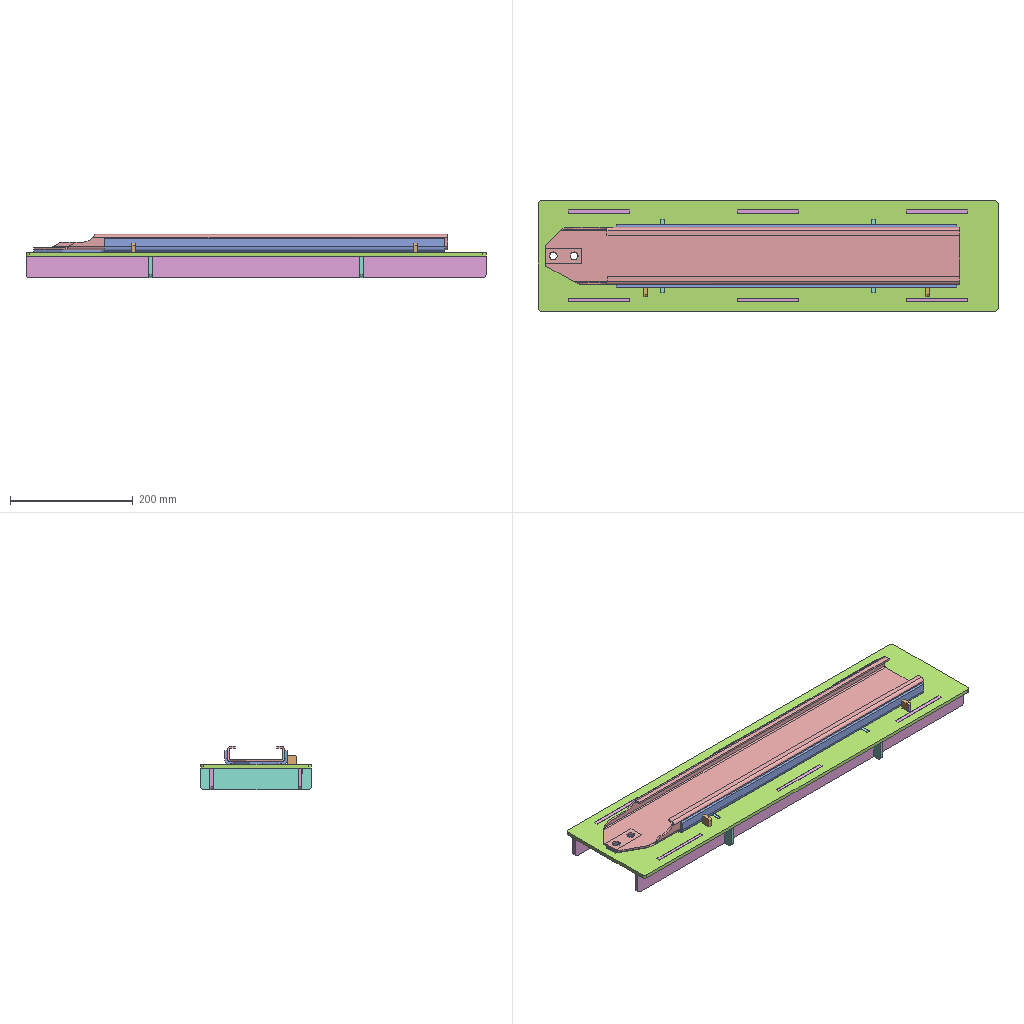Assembly | SolidWorks | 7 different items | 10 placed | box 750 x 180 x 70 mm
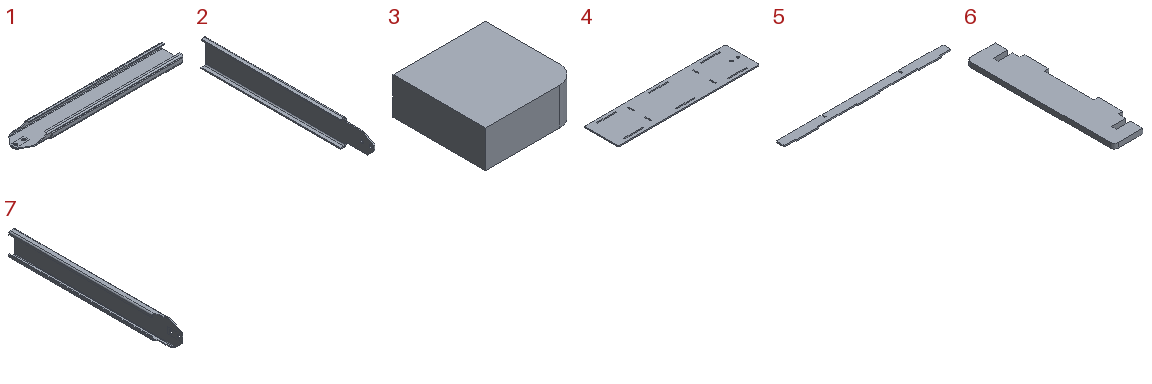Parts list (item | name | quantity | parent item | size | volume | features):
1 | (subassembly) | x1 | - | 675 x 102.2 x 29.4 mm | 664944 mm3 | -
2 | - | x1 | in 1 | 22.5 x 670 x 102.2 mm | 361914 mm3 | features ICE 2, FlatPattern 1, SMBaseFlange 1, SheetMetal 1
3 | - | x2 | - | 15 x 15 x 6 mm | 1338 mm3 | features FlatPattern 1, SMBaseFlange 1, SheetMetal 1
4 | - | x1 | - | 750 x 180 x 6 mm | 782502 mm3 | features FlatPattern 1, SMBaseFlange 1, SheetMetal 1
5 | - | x2 | - | 750 x 40.5 x 6 mm | 166068 mm3 | features FlatPattern 1, SMBaseFlange 1, SheetMetal 1
6 | - | x2 | - | 40.5 x 180 x 6 mm | 38456 mm3 | features FlatPattern 1, SMBaseFlange 1, SheetMetal 1
7 | - | x1 | in 1 | 24.9 x 675 x 92.9 mm | 303030 mm3 | features ICE 4, FlatPattern 1, SMBaseFlange 1, SheetMetal 1
Mates (type | each side: item.copy, entity, surface, feature):
In the top assembly
InPlace | 5.1 plane | assembly plane
InPlace | 6.1 plane | assembly plane
In subassembly 1
Coincident | 7.1 face plane Base-Flange1 | 2.1 face plane Base-Flange1 | 2 times
Concentric | 7.1 face cylinder Cut-Extrude5 | 2.1 face cylinder Cut-Extrude1 | 2 times